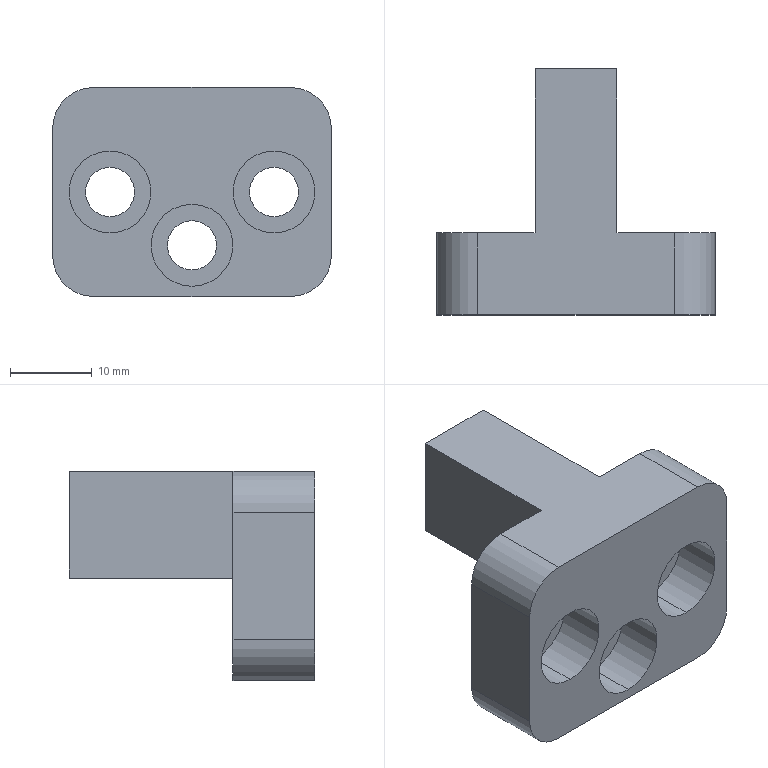Part | STEP file | 1 solid | 29 faces | box 34 x 30 x 25.5 mm | volume 9302 mm3 | cylinder 16 | plane 13 | commonest cylinder face diameters 10 x10 6 x6